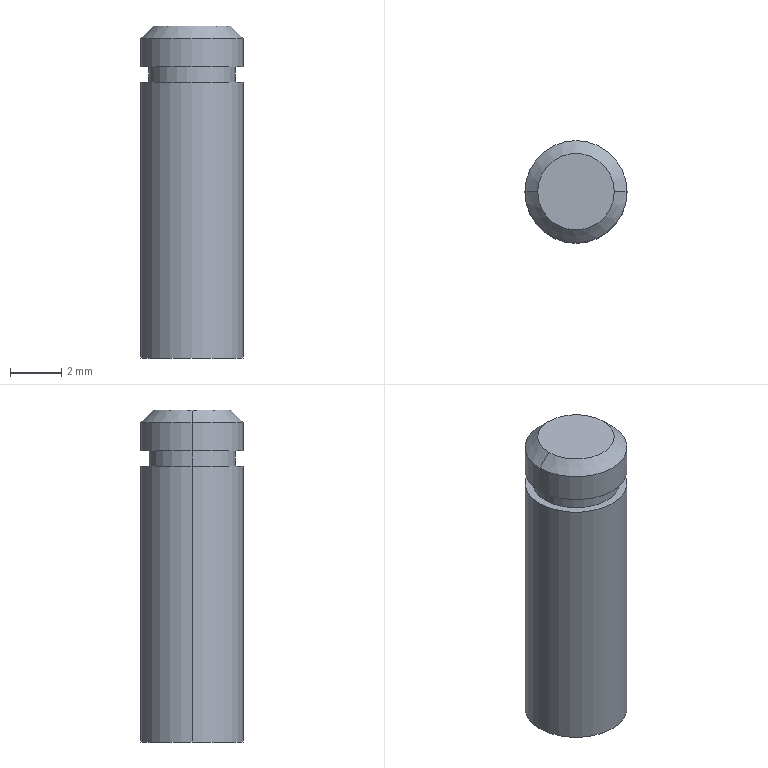Part | SolidWorks | features ICE 2, Chamfer 1, Extrusion 1 | 1 solid | 12 faces | box 4 x 4 x 13 mm | volume 159.831 mm3 | cylinder 6 | plane 4 | cone 2 | commonest cylinder face diameters 4 x4 3.4 x2
STEP:
#1=CARTESIAN_POINT('',(1.5,0.,13.));
#2=VERTEX_POINT('',#1);
#3=CARTESIAN_POINT('',(-1.5,0.,13.));
#4=VERTEX_POINT('',#3);
#5=CARTESIAN_POINT('',(0.,0.,13.));
#6=DIRECTION('',(0.,0.,1.));
#7=DIRECTION('',(1.,0.,0.));
#8=AXIS2_PLACEMENT_3D('',#5,#6,#7);
#9=CIRCLE('',#8,1.5);
#10=EDGE_CURVE('',#2,#4,#9,.T.);
#11=ORIENTED_EDGE('',*,*,#10,.F.);
#12=CARTESIAN_POINT('',(2.,0.,12.5));
#13=VERTEX_POINT('',#12);
#14=CARTESIAN_POINT('',(1.5,0.,13.));
#15=DIRECTION('',(0.7071,0.,-0.7071));
#16=VECTOR('',#15,1000.);
#17=LINE('',#14,#16);
#18=EDGE_CURVE('',#2,#13,#17,.T.);
#19=ORIENTED_EDGE('',*,*,#18,.T.);
#20=CARTESIAN_POINT('',(-2.,0.,12.5));
#21=VERTEX_POINT('',#20);
#22=CARTESIAN_POINT('',(0.,0.,12.5));
#23=DIRECTION('',(0.,0.,-1.));
#24=DIRECTION('',(1.,0.,0.));
#25=AXIS2_PLACEMENT_3D('',#22,#23,#24);
#26=CIRCLE('',#25,2.);
#27=EDGE_CURVE('',#21,#13,#26,.T.);
#28=ORIENTED_EDGE('',*,*,#27,.F.);
#29=CARTESIAN_POINT('',(-1.5,0.,13.));
#30=DIRECTION('',(-0.7071,0.,-0.7071));
#31=VECTOR('',#30,1000.);
#32=LINE('',#29,#31);
#33=EDGE_CURVE('',#4,#21,#32,.T.);
#34=ORIENTED_EDGE('',*,*,#33,.F.);
#35=EDGE_LOOP('',(#11,#19,#28,#34));
#36=FACE_OUTER_BOUND('',#35,.T.);
#37=CARTESIAN_POINT('',(0.,0.,13.));
#38=DIRECTION('',(0.,0.,-1.));
#39=DIRECTION('',(-1.,0.,0.));
#40=AXIS2_PLACEMENT_3D('',#37,#38,#39);
#41=CONICAL_SURFACE('',#40,1.5,0.7854);
#42=ADVANCED_FACE('',(#36),#41,.T.);
#43=ORIENTED_EDGE('',*,*,#27,.T.);
#44=CARTESIAN_POINT('',(2.,0.,11.4));
#45=VERTEX_POINT('',#44);
#46=CARTESIAN_POINT('',(2.,0.,13.));
#47=DIRECTION('',(0.,0.,-1.));
#48=VECTOR('',#47,1000.);
#49=LINE('',#46,#48);
#50=EDGE_CURVE('',#13,#45,#49,.T.);
#51=ORIENTED_EDGE('',*,*,#50,.T.);
#52=CARTESIAN_POINT('',(-2.,0.,11.4));
#53=VERTEX_POINT('',#52);
#54=CARTESIAN_POINT('',(0.,0.,11.4));
#55=DIRECTION('',(0.,0.,1.));
#56=DIRECTION('',(1.,0.,0.));
#57=AXIS2_PLACEMENT_3D('',#54,#55,#56);
#58=CIRCLE('',#57,2.);
#59=EDGE_CURVE('',#45,#53,#58,.T.);
#60=ORIENTED_EDGE('',*,*,#59,.T.);
#61=CARTESIAN_POINT('',(-2.,0.,13.));
#62=DIRECTION('',(0.,0.,-1.));
#63=VECTOR('',#62,1000.);
#64=LINE('',#61,#63);
#65=EDGE_CURVE('',#21,#53,#64,.T.);
#66=ORIENTED_EDGE('',*,*,#65,.F.);
#67=EDGE_LOOP('',(#43,#51,#60,#66));
#68=FACE_OUTER_BOUND('',#67,.T.);
#69=CARTESIAN_POINT('',(0.,0.,13.));
#70=DIRECTION('',(0.,0.,-1.));
#71=DIRECTION('',(-1.,0.,0.));
#72=AXIS2_PLACEMENT_3D('',#69,#70,#71);
#73=CYLINDRICAL_SURFACE('',#72,2.);
#74=ADVANCED_FACE('',(#68),#73,.T.);
#75=CARTESIAN_POINT('',(1.7,0.,11.4));
#76=VERTEX_POINT('',#75);
#77=CARTESIAN_POINT('',(-1.7,0.,11.4));
#78=VERTEX_POINT('',#77);
#79=CARTESIAN_POINT('',(0.,0.,11.4));
#80=DIRECTION('',(0.,0.,1.));
#81=DIRECTION('',(1.,0.,0.));
#82=AXIS2_PLACEMENT_3D('',#79,#80,#81);
#83=CIRCLE('',#82,1.7);
#84=EDGE_CURVE('',#76,#78,#83,.T.);
#85=ORIENTED_EDGE('',*,*,#84,.F.);
#86=CARTESIAN_POINT('',(1.7,0.,10.8));
#87=VERTEX_POINT('',#86);
#88=CARTESIAN_POINT('',(1.7,0.,11.4));
#89=DIRECTION('',(0.,0.,-1.));
#90=VECTOR('',#89,1000.);
#91=LINE('',#88,#90);
#92=EDGE_CURVE('',#76,#87,#91,.T.);
#93=ORIENTED_EDGE('',*,*,#92,.T.);
#94=CARTESIAN_POINT('',(-1.7,0.,10.8));
#95=VERTEX_POINT('',#94);
#96=CARTESIAN_POINT('',(0.,0.,10.8));
#97=DIRECTION('',(0.,0.,1.));
#98=DIRECTION('',(1.,0.,0.));
#99=AXIS2_PLACEMENT_3D('',#96,#97,#98);
#100=CIRCLE('',#99,1.7);
#101=EDGE_CURVE('',#87,#95,#100,.T.);
#102=ORIENTED_EDGE('',*,*,#101,.T.);
#103=CARTESIAN_POINT('',(-1.7,0.,11.4));
#104=DIRECTION('',(0.,0.,-1.));
#105=VECTOR('',#104,1000.);
#106=LINE('',#103,#105);
#107=EDGE_CURVE('',#78,#95,#106,.T.);
#108=ORIENTED_EDGE('',*,*,#107,.F.);
#109=EDGE_LOOP('',(#85,#93,#102,#108));
#110=FACE_OUTER_BOUND('',#109,.T.);
#111=CARTESIAN_POINT('',(0.,0.,11.4));
#112=DIRECTION('',(0.,0.,-1.));
#113=DIRECTION('',(-1.,0.,0.));
#114=AXIS2_PLACEMENT_3D('',#111,#112,#113);
#115=CYLINDRICAL_SURFACE('',#114,1.7);
#116=ADVANCED_FACE('',(#110),#115,.T.);
#117=CARTESIAN_POINT('',(2.,0.,10.8));
#118=VERTEX_POINT('',#117);
#119=CARTESIAN_POINT('',(-2.,0.,10.8));
#120=VERTEX_POINT('',#119);
#121=CARTESIAN_POINT('',(0.,0.,10.8));
#122=DIRECTION('',(0.,0.,1.));
#123=DIRECTION('',(1.,0.,0.));
#124=AXIS2_PLACEMENT_3D('',#121,#122,#123);
#125=CIRCLE('',#124,2.);
#126=EDGE_CURVE('',#118,#120,#125,.T.);
#127=ORIENTED_EDGE('',*,*,#126,.F.);
#128=CARTESIAN_POINT('',(2.,0.,0.));
#129=VERTEX_POINT('',#128);
#130=CARTESIAN_POINT('',(2.,0.,10.8));
#131=DIRECTION('',(0.,0.,-1.));
#132=VECTOR('',#131,1000.);
#133=LINE('',#130,#132);
#134=EDGE_CURVE('',#118,#129,#133,.T.);
#135=ORIENTED_EDGE('',*,*,#134,.T.);
#136=CARTESIAN_POINT('',(-2.,0.,0.));
#137=VERTEX_POINT('',#136);
#138=CARTESIAN_POINT('',(0.,0.,0.));
#139=DIRECTION('',(0.,0.,1.));
#140=DIRECTION('',(1.,0.,0.));
#141=AXIS2_PLACEMENT_3D('',#138,#139,#140);
#142=CIRCLE('',#141,2.);
#143=EDGE_CURVE('',#129,#137,#142,.T.);
#144=ORIENTED_EDGE('',*,*,#143,.T.);
#145=CARTESIAN_POINT('',(-2.,0.,10.8));
#146=DIRECTION('',(0.,0.,-1.));
#147=VECTOR('',#146,1000.);
#148=LINE('',#145,#147);
#149=EDGE_CURVE('',#120,#137,#148,.T.);
#150=ORIENTED_EDGE('',*,*,#149,.F.);
#151=EDGE_LOOP('',(#127,#135,#144,#150));
#152=FACE_OUTER_BOUND('',#151,.T.);
#153=CARTESIAN_POINT('',(0.,0.,10.8));
#154=DIRECTION('',(0.,0.,-1.));
#155=DIRECTION('',(-1.,0.,0.));
#156=AXIS2_PLACEMENT_3D('',#153,#154,#155);
#157=CYLINDRICAL_SURFACE('',#156,2.);
#158=ADVANCED_FACE('',(#152),#157,.T.);
#159=ORIENTED_EDGE('',*,*,#134,.F.);
#160=CARTESIAN_POINT('',(0.,0.,10.8));
#161=DIRECTION('',(0.,0.,1.));
#162=DIRECTION('',(1.,0.,0.));
#163=AXIS2_PLACEMENT_3D('',#160,#161,#162);
#164=CIRCLE('',#163,2.);
#165=EDGE_CURVE('',#120,#118,#164,.T.);
#166=ORIENTED_EDGE('',*,*,#165,.F.);
#167=ORIENTED_EDGE('',*,*,#149,.T.);
#168=CARTESIAN_POINT('',(0.,0.,0.));
#169=DIRECTION('',(0.,0.,1.));
#170=DIRECTION('',(1.,0.,0.));
#171=AXIS2_PLACEMENT_3D('',#168,#169,#170);
#172=CIRCLE('',#171,2.);
#173=EDGE_CURVE('',#137,#129,#172,.T.);
#174=ORIENTED_EDGE('',*,*,#173,.T.);
#175=EDGE_LOOP('',(#159,#166,#167,#174));
#176=FACE_OUTER_BOUND('',#175,.T.);
#177=CARTESIAN_POINT('',(0.,0.,10.8));
#178=DIRECTION('',(0.,0.,-1.));
#179=DIRECTION('',(-1.,0.,0.));
#180=AXIS2_PLACEMENT_3D('',#177,#178,#179);
#181=CYLINDRICAL_SURFACE('',#180,2.);
#182=ADVANCED_FACE('',(#176),#181,.T.);
#183=CARTESIAN_POINT('',(0.,0.,10.8));
#184=DIRECTION('',(0.,0.,1.));
#185=DIRECTION('',(1.,0.,0.));
#186=AXIS2_PLACEMENT_3D('',#183,#184,#185);
#187=CIRCLE('',#186,1.7);
#188=EDGE_CURVE('',#95,#87,#187,.T.);
#189=ORIENTED_EDGE('',*,*,#188,.F.);
#190=ORIENTED_EDGE('',*,*,#101,.F.);
#191=EDGE_LOOP('',(#189,#190));
#192=FACE_BOUND('',#191,.T.);
#193=ORIENTED_EDGE('',*,*,#165,.T.);
#194=ORIENTED_EDGE('',*,*,#126,.T.);
#195=EDGE_LOOP('',(#193,#194));
#196=FACE_OUTER_BOUND('',#195,.T.);
#197=CARTESIAN_POINT('',(0.,0.,10.8));
#198=DIRECTION('',(0.,0.,1.));
#199=DIRECTION('',(1.,0.,0.));
#200=AXIS2_PLACEMENT_3D('',#197,#198,#199);
#201=PLANE('',#200);
#202=ADVANCED_FACE('',(#192,#196),#201,.T.);
#203=ORIENTED_EDGE('',*,*,#173,.F.);
#204=ORIENTED_EDGE('',*,*,#143,.F.);
#205=EDGE_LOOP('',(#203,#204));
#206=FACE_OUTER_BOUND('',#205,.T.);
#207=CARTESIAN_POINT('',(0.,0.,0.));
#208=DIRECTION('',(0.,0.,1.));
#209=DIRECTION('',(1.,0.,0.));
#210=AXIS2_PLACEMENT_3D('',#207,#208,#209);
#211=PLANE('',#210);
#212=ADVANCED_FACE('',(#206),#211,.F.);
#213=ORIENTED_EDGE('',*,*,#92,.F.);
#214=CARTESIAN_POINT('',(0.,0.,11.4));
#215=DIRECTION('',(0.,0.,1.));
#216=DIRECTION('',(1.,0.,0.));
#217=AXIS2_PLACEMENT_3D('',#214,#215,#216);
#218=CIRCLE('',#217,1.7);
#219=EDGE_CURVE('',#78,#76,#218,.T.);
#220=ORIENTED_EDGE('',*,*,#219,.F.);
#221=ORIENTED_EDGE('',*,*,#107,.T.);
#222=ORIENTED_EDGE('',*,*,#188,.T.);
#223=EDGE_LOOP('',(#213,#220,#221,#222));
#224=FACE_OUTER_BOUND('',#223,.T.);
#225=CARTESIAN_POINT('',(0.,0.,11.4));
#226=DIRECTION('',(0.,0.,-1.));
#227=DIRECTION('',(-1.,0.,0.));
#228=AXIS2_PLACEMENT_3D('',#225,#226,#227);
#229=CYLINDRICAL_SURFACE('',#228,1.7);
#230=ADVANCED_FACE('',(#224),#229,.T.);
#231=ORIENTED_EDGE('',*,*,#50,.F.);
#232=CARTESIAN_POINT('',(0.,0.,12.5));
#233=DIRECTION('',(0.,0.,-1.));
#234=DIRECTION('',(1.,0.,0.));
#235=AXIS2_PLACEMENT_3D('',#232,#233,#234);
#236=CIRCLE('',#235,2.);
#237=EDGE_CURVE('',#13,#21,#236,.T.);
#238=ORIENTED_EDGE('',*,*,#237,.T.);
#239=ORIENTED_EDGE('',*,*,#65,.T.);
#240=CARTESIAN_POINT('',(0.,0.,11.4));
#241=DIRECTION('',(0.,0.,1.));
#242=DIRECTION('',(1.,0.,0.));
#243=AXIS2_PLACEMENT_3D('',#240,#241,#242);
#244=CIRCLE('',#243,2.);
#245=EDGE_CURVE('',#53,#45,#244,.T.);
#246=ORIENTED_EDGE('',*,*,#245,.T.);
#247=EDGE_LOOP('',(#231,#238,#239,#246));
#248=FACE_OUTER_BOUND('',#247,.T.);
#249=CARTESIAN_POINT('',(0.,0.,13.));
#250=DIRECTION('',(0.,0.,-1.));
#251=DIRECTION('',(-1.,0.,0.));
#252=AXIS2_PLACEMENT_3D('',#249,#250,#251);
#253=CYLINDRICAL_SURFACE('',#252,2.);
#254=ADVANCED_FACE('',(#248),#253,.T.);
#255=CARTESIAN_POINT('',(0.,0.,13.));
#256=DIRECTION('',(0.,0.,1.));
#257=DIRECTION('',(1.,0.,0.));
#258=AXIS2_PLACEMENT_3D('',#255,#256,#257);
#259=CIRCLE('',#258,1.5);
#260=EDGE_CURVE('',#4,#2,#259,.T.);
#261=ORIENTED_EDGE('',*,*,#260,.T.);
#262=ORIENTED_EDGE('',*,*,#10,.T.);
#263=EDGE_LOOP('',(#261,#262));
#264=FACE_OUTER_BOUND('',#263,.T.);
#265=CARTESIAN_POINT('',(0.,0.,13.));
#266=DIRECTION('',(0.,0.,1.));
#267=DIRECTION('',(1.,0.,0.));
#268=AXIS2_PLACEMENT_3D('',#265,#266,#267);
#269=PLANE('',#268);
#270=ADVANCED_FACE('',(#264),#269,.T.);
#271=ORIENTED_EDGE('',*,*,#219,.T.);
#272=ORIENTED_EDGE('',*,*,#84,.T.);
#273=EDGE_LOOP('',(#271,#272));
#274=FACE_BOUND('',#273,.T.);
#275=ORIENTED_EDGE('',*,*,#245,.F.);
#276=ORIENTED_EDGE('',*,*,#59,.F.);
#277=EDGE_LOOP('',(#275,#276));
#278=FACE_OUTER_BOUND('',#277,.T.);
#279=CARTESIAN_POINT('',(0.,0.,11.4));
#280=DIRECTION('',(0.,0.,1.));
#281=DIRECTION('',(1.,0.,0.));
#282=AXIS2_PLACEMENT_3D('',#279,#280,#281);
#283=PLANE('',#282);
#284=ADVANCED_FACE('',(#274,#278),#283,.F.);
#285=ORIENTED_EDGE('',*,*,#18,.F.);
#286=ORIENTED_EDGE('',*,*,#260,.F.);
#287=ORIENTED_EDGE('',*,*,#33,.T.);
#288=ORIENTED_EDGE('',*,*,#237,.F.);
#289=EDGE_LOOP('',(#285,#286,#287,#288));
#290=FACE_OUTER_BOUND('',#289,.T.);
#291=CARTESIAN_POINT('',(0.,0.,13.));
#292=DIRECTION('',(0.,0.,-1.));
#293=DIRECTION('',(-1.,0.,0.));
#294=AXIS2_PLACEMENT_3D('',#291,#292,#293);
#295=CONICAL_SURFACE('',#294,1.5,0.7854);
#296=ADVANCED_FACE('',(#290),#295,.T.);
#297=CLOSED_SHELL('',(#42,#74,#116,#158,#182,#202,#212,#230,#254,#270,#284,#296));
#298=MANIFOLD_SOLID_BREP('',#297);
#299=CARTESIAN_POINT('',(0.,0.,0.));
#300=DIRECTION('',(0.,0.,1.));
#301=DIRECTION('',(1.,0.,0.));
#302=AXIS2_PLACEMENT_3D('',#299,#300,#301);
#303=(LENGTH_UNIT()NAMED_UNIT(*)SI_UNIT(.MILLI.,.METRE.));
#304=UNCERTAINTY_MEASURE_WITH_UNIT(LENGTH_MEASURE(0.00001),#303,'','');
#305=(NAMED_UNIT(*)PLANE_ANGLE_UNIT()SI_UNIT($,.RADIAN.));
#306=(NAMED_UNIT(*)SI_UNIT($,.STERADIAN.)SOLID_ANGLE_UNIT());
#307=(GEOMETRIC_REPRESENTATION_CONTEXT(3)GLOBAL_UNCERTAINTY_ASSIGNED_CONTEXT((#304))GLOBAL_UNIT_ASSIGNED_CONTEXT((#303,#305,#306))REPRESENTATION_CONTEXT('',''));
#308=ADVANCED_BREP_SHAPE_REPRESENTATION('',(#298,#302),#307);